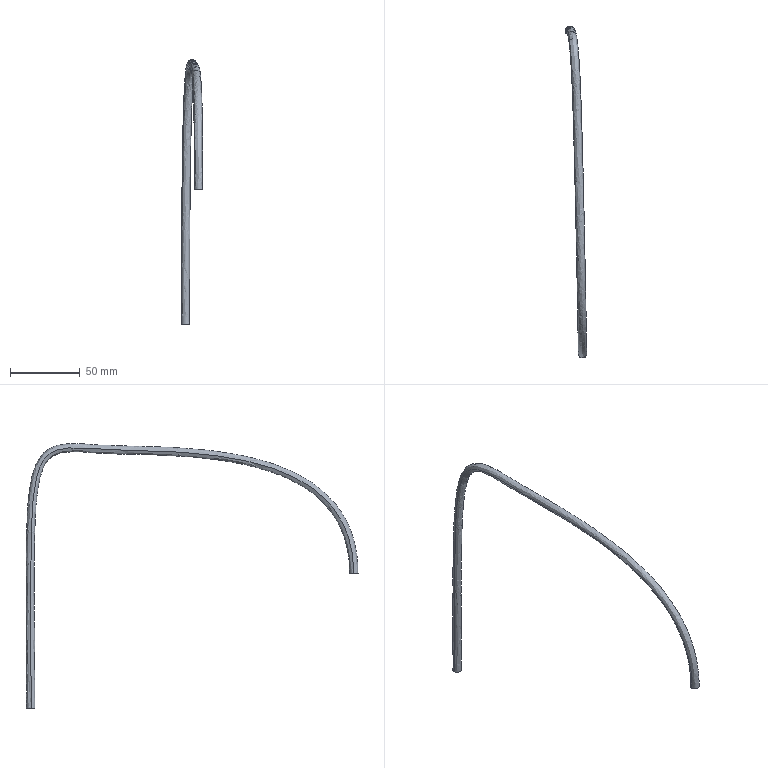Part | SolidWorks | features BaseBody 1 | 1 solid | 4 faces | box 15.406 x 237.723 x 189.724 mm | volume 12762 mm3 | spline 2 | plane 2
STEP:
#1=CARTESIAN_POINT('',(602.943,-193.052,343.045));
#2=VERTEX_POINT('',#1);
#3=CARTESIAN_POINT('',(596.944,-193.051,343.045));
#4=VERTEX_POINT('',#3);
#5=CARTESIAN_POINT('',(602.943,-193.052,343.045));
#6=CARTESIAN_POINT('',(602.943,-192.266,343.045));
#7=CARTESIAN_POINT('',(602.293,-190.702,343.045));
#8=CARTESIAN_POINT('',(599.943,-189.728,343.045));
#9=CARTESIAN_POINT('',(597.593,-190.702,343.045));
#10=CARTESIAN_POINT('',(596.944,-192.268,343.045));
#11=CARTESIAN_POINT('',(596.944,-193.051,343.045));
#12=B_SPLINE_CURVE_WITH_KNOTS('',3,(#5,#6,#7,#8,#9,#10,#11),.UNSPECIFIED.,.F.,.F.,(4,1,1,1,4),(0.009368,0.01171,0.01405,0.0164,0.01874),.UNSPECIFIED.);
#13=EDGE_CURVE('',#2,#4,#12,.T.);
#14=ORIENTED_EDGE('',*,*,#13,.T.);
#15=CARTESIAN_POINT('',(587.558,37.99,246.432));
#16=VERTEX_POINT('',#15);
#17=CARTESIAN_POINT('',(596.944,-193.051,343.045));
#18=CARTESIAN_POINT('',(596.944,-193.048,355.466));
#19=CARTESIAN_POINT('',(596.907,-190.885,366.117));
#20=CARTESIAN_POINT('',(596.772,-183.095,384.368));
#21=CARTESIAN_POINT('',(596.672,-177.485,391.983));
#22=CARTESIAN_POINT('',(596.422,-163.694,404.684));
#23=CARTESIAN_POINT('',(596.119,-147.351,414.874));
#24=CARTESIAN_POINT('',(595.344,-107.987,427.25));
#25=CARTESIAN_POINT('',(594.381,-63.958,430.712));
#26=CARTESIAN_POINT('',(593.449,-29.528,431.39));
#27=CARTESIAN_POINT('',(592.967,-14.614,431.839));
#28=CARTESIAN_POINT('',(592.728,-8.166,432.222));
#29=CARTESIAN_POINT('',(592.641,-5.946,432.39));
#30=CARTESIAN_POINT('',(592.61,-5.155,432.454));
#31=CARTESIAN_POINT('',(592.594,-4.765,432.487));
#32=CARTESIAN_POINT('',(592.334,1.621,433.044));
#33=CARTESIAN_POINT('',(591.933,9.581,433.39));
#34=CARTESIAN_POINT('',(591.378,17.891,432.117));
#35=CARTESIAN_POINT('',(590.956,23.07,430.097));
#36=CARTESIAN_POINT('',(590.535,27.306,426.808));
#37=CARTESIAN_POINT('',(590.118,30.703,422.03));
#38=CARTESIAN_POINT('',(589.575,34.228,413.383));
#39=CARTESIAN_POINT('',(589.193,35.866,404.037));
#40=CARTESIAN_POINT('',(588.607,37.778,384.601));
#41=CARTESIAN_POINT('',(588.299,38.193,369.487));
#42=CARTESIAN_POINT('',(587.905,38.355,336.976));
#43=CARTESIAN_POINT('',(587.652,38.205,307.087));
#44=CARTESIAN_POINT('',(587.558,37.99,268.306));
#45=CARTESIAN_POINT('',(587.558,37.99,246.432));
#46=B_SPLINE_CURVE_WITH_KNOTS('',3,(#17,#18,#19,#20,#21,#22,#23,#24,#25,#26,#27,#28,#29,#30,#31,#32,#33,#34,#35,#36,#37,#38,#39,#40,#41,#42,#43,#44,#45),.UNSPECIFIED.,.F.,.F.,(4,2,2,1,1,1,1,1,1,1,1,2,1,1,1,1,1,1,2,2,1,4),(0.,0.0625,0.125,0.1875,0.25,0.375,0.4375,0.4766,0.4922,0.4961,0.498,0.5,0.5625,0.5938,0.625,0.6562,0.6875,0.7188,0.7812,0.875,0.9375,1.),.UNSPECIFIED.);
#47=EDGE_CURVE('',#4,#16,#46,.T.);
#48=ORIENTED_EDGE('',*,*,#47,.T.);
#49=CARTESIAN_POINT('',(593.513,38.709,246.432));
#50=VERTEX_POINT('',#49);
#51=CARTESIAN_POINT('',(587.558,37.99,246.432));
#52=CARTESIAN_POINT('',(587.652,37.212,246.432));
#53=CARTESIAN_POINT('',(588.484,35.735,246.432));
#54=CARTESIAN_POINT('',(590.934,35.05,246.432));
#55=CARTESIAN_POINT('',(593.15,36.298,246.432));
#56=CARTESIAN_POINT('',(593.608,37.93,246.432));
#57=CARTESIAN_POINT('',(593.513,38.709,246.432));
#58=B_SPLINE_CURVE_WITH_KNOTS('',3,(#51,#52,#53,#54,#55,#56,#57),.UNSPECIFIED.,.F.,.F.,(4,1,1,1,4),(0.009368,0.01171,0.01405,0.0164,0.01874),.UNSPECIFIED.);
#59=EDGE_CURVE('',#16,#50,#58,.T.);
#60=ORIENTED_EDGE('',*,*,#59,.T.);
#61=CARTESIAN_POINT('',(602.943,-193.052,343.045));
#62=CARTESIAN_POINT('',(602.943,-193.048,355.478));
#63=CARTESIAN_POINT('',(602.906,-190.883,366.144));
#64=CARTESIAN_POINT('',(602.77,-183.081,384.424));
#65=CARTESIAN_POINT('',(602.671,-177.461,392.052));
#66=CARTESIAN_POINT('',(602.42,-163.647,404.773));
#67=CARTESIAN_POINT('',(602.116,-147.282,414.978));
#68=CARTESIAN_POINT('',(601.341,-107.88,427.364));
#69=CARTESIAN_POINT('',(600.377,-63.823,430.829));
#70=CARTESIAN_POINT('',(599.444,-29.358,431.508));
#71=CARTESIAN_POINT('',(598.961,-14.416,431.957));
#72=CARTESIAN_POINT('',(598.722,-7.948,432.341));
#73=CARTESIAN_POINT('',(598.635,-5.719,432.51));
#74=CARTESIAN_POINT('',(598.603,-4.925,432.574));
#75=CARTESIAN_POINT('',(598.587,-4.533,432.608));
#76=CARTESIAN_POINT('',(598.326,1.89,433.168));
#77=CARTESIAN_POINT('',(597.922,9.916,433.52));
#78=CARTESIAN_POINT('',(597.358,18.357,432.229));
#79=CARTESIAN_POINT('',(596.927,23.646,430.168));
#80=CARTESIAN_POINT('',(596.497,27.97,426.809));
#81=CARTESIAN_POINT('',(596.074,31.409,421.965));
#82=CARTESIAN_POINT('',(595.529,34.951,413.27));
#83=CARTESIAN_POINT('',(595.148,36.587,403.924));
#84=CARTESIAN_POINT('',(594.561,38.498,384.498));
#85=CARTESIAN_POINT('',(594.254,38.912,369.401));
#86=CARTESIAN_POINT('',(593.86,39.075,336.919));
#87=CARTESIAN_POINT('',(593.608,38.925,307.053));
#88=CARTESIAN_POINT('',(593.514,38.71,268.295));
#89=CARTESIAN_POINT('',(593.513,38.709,246.432));
#90=B_SPLINE_CURVE_WITH_KNOTS('',3,(#61,#62,#63,#64,#65,#66,#67,#68,#69,#70,#71,#72,#73,#74,#75,#76,#77,#78,#79,#80,#81,#82,#83,#84,#85,#86,#87,#88,#89),.UNSPECIFIED.,.F.,.F.,(4,2,2,1,1,1,1,1,1,1,1,2,1,1,1,1,1,1,2,2,1,4),(0.,0.0625,0.125,0.1875,0.25,0.375,0.4375,0.4766,0.4922,0.4961,0.498,0.5,0.5625,0.5938,0.625,0.6562,0.6875,0.7188,0.7812,0.875,0.9375,1.),.UNSPECIFIED.);
#91=EDGE_CURVE('',#2,#50,#90,.T.);
#92=ORIENTED_EDGE('',*,*,#91,.F.);
#93=EDGE_LOOP('',(#14,#48,#60,#92));
#94=FACE_OUTER_BOUND('',#93,.T.);
#95=CARTESIAN_POINT('',(602.943,-193.052,343.045));
#96=CARTESIAN_POINT('',(602.943,-193.048,355.478));
#97=CARTESIAN_POINT('',(602.906,-190.883,366.144));
#98=CARTESIAN_POINT('',(602.77,-183.081,384.424));
#99=CARTESIAN_POINT('',(602.671,-177.461,392.052));
#100=CARTESIAN_POINT('',(602.42,-163.647,404.773));
#101=CARTESIAN_POINT('',(602.116,-147.282,414.978));
#102=CARTESIAN_POINT('',(601.341,-107.88,427.364));
#103=CARTESIAN_POINT('',(600.377,-63.823,430.829));
#104=CARTESIAN_POINT('',(599.444,-29.358,431.508));
#105=CARTESIAN_POINT('',(598.961,-14.416,431.957));
#106=CARTESIAN_POINT('',(598.722,-7.948,432.341));
#107=CARTESIAN_POINT('',(598.635,-5.719,432.51));
#108=CARTESIAN_POINT('',(598.603,-4.925,432.574));
#109=CARTESIAN_POINT('',(598.587,-4.533,432.608));
#110=CARTESIAN_POINT('',(598.326,1.89,433.168));
#111=CARTESIAN_POINT('',(597.922,9.916,433.52));
#112=CARTESIAN_POINT('',(597.358,18.357,432.229));
#113=CARTESIAN_POINT('',(596.927,23.646,430.168));
#114=CARTESIAN_POINT('',(596.497,27.97,426.809));
#115=CARTESIAN_POINT('',(596.074,31.409,421.965));
#116=CARTESIAN_POINT('',(595.529,34.951,413.27));
#117=CARTESIAN_POINT('',(595.148,36.587,403.924));
#118=CARTESIAN_POINT('',(594.561,38.498,384.498));
#119=CARTESIAN_POINT('',(594.254,38.912,369.401));
#120=CARTESIAN_POINT('',(593.86,39.075,336.919));
#121=CARTESIAN_POINT('',(593.608,38.925,307.053));
#122=CARTESIAN_POINT('',(593.514,38.71,268.295));
#123=CARTESIAN_POINT('',(593.513,38.709,246.432));
#124=CARTESIAN_POINT('',(602.943,-192.266,343.045));
#125=CARTESIAN_POINT('',(602.943,-192.263,355.386));
#126=CARTESIAN_POINT('',(602.907,-190.115,365.941));
#127=CARTESIAN_POINT('',(602.772,-182.404,384.01));
#128=CARTESIAN_POINT('',(602.674,-176.855,391.543));
#129=CARTESIAN_POINT('',(602.425,-163.189,404.128));
#130=CARTESIAN_POINT('',(602.125,-146.968,414.249));
#131=CARTESIAN_POINT('',(601.354,-107.762,426.581));
#132=CARTESIAN_POINT('',(600.392,-63.79,430.044));
#133=CARTESIAN_POINT('',(599.459,-29.344,430.723));
#134=CARTESIAN_POINT('',(598.976,-14.385,431.172));
#135=CARTESIAN_POINT('',(598.736,-7.896,431.558));
#136=CARTESIAN_POINT('',(598.648,-5.658,431.727));
#137=CARTESIAN_POINT('',(598.616,-4.86,431.792));
#138=CARTESIAN_POINT('',(598.6,-4.464,431.826));
#139=CARTESIAN_POINT('',(598.34,1.94,432.384));
#140=CARTESIAN_POINT('',(597.938,9.912,432.729));
#141=CARTESIAN_POINT('',(597.386,18.17,431.46));
#142=CARTESIAN_POINT('',(596.971,23.264,429.47));
#143=CARTESIAN_POINT('',(596.56,27.392,426.263));
#144=CARTESIAN_POINT('',(596.153,30.712,421.598));
#145=CARTESIAN_POINT('',(595.618,34.184,413.089));
#146=CARTESIAN_POINT('',(595.239,35.815,403.813));
#147=CARTESIAN_POINT('',(594.655,37.717,384.467));
#148=CARTESIAN_POINT('',(594.348,38.133,369.387));
#149=CARTESIAN_POINT('',(593.954,38.295,336.92));
#150=CARTESIAN_POINT('',(593.702,38.145,307.059));
#151=CARTESIAN_POINT('',(593.608,37.93,268.298));
#152=CARTESIAN_POINT('',(593.608,37.93,246.432));
#153=CARTESIAN_POINT('',(602.293,-190.702,343.045));
#154=CARTESIAN_POINT('',(602.293,-190.698,355.203));
#155=CARTESIAN_POINT('',(602.257,-188.586,365.536));
#156=CARTESIAN_POINT('',(602.126,-181.056,383.18));
#157=CARTESIAN_POINT('',(602.03,-175.651,390.52));
#158=CARTESIAN_POINT('',(601.787,-162.28,402.833));
#159=CARTESIAN_POINT('',(601.492,-146.352,412.786));
#160=CARTESIAN_POINT('',(600.729,-107.538,425.007));
#161=CARTESIAN_POINT('',(599.771,-63.74,428.469));
#162=CARTESIAN_POINT('',(598.84,-29.334,429.146));
#163=CARTESIAN_POINT('',(598.355,-14.346,429.596));
#164=CARTESIAN_POINT('',(598.114,-7.817,429.984));
#165=CARTESIAN_POINT('',(598.025,-5.559,430.155));
#166=CARTESIAN_POINT('',(597.993,-4.756,430.22));
#167=CARTESIAN_POINT('',(597.977,-4.351,430.254));
#168=CARTESIAN_POINT('',(597.718,2.011,430.809));
#169=CARTESIAN_POINT('',(597.321,9.868,431.138));
#170=CARTESIAN_POINT('',(596.793,17.749,429.916));
#171=CARTESIAN_POINT('',(596.411,22.44,428.071));
#172=CARTESIAN_POINT('',(596.04,26.169,425.175));
#173=CARTESIAN_POINT('',(595.663,29.245,420.873));
#174=CARTESIAN_POINT('',(595.151,32.579,412.74));
#175=CARTESIAN_POINT('',(594.776,34.197,403.603));
#176=CARTESIAN_POINT('',(594.197,36.084,384.416));
#177=CARTESIAN_POINT('',(593.89,36.501,369.368));
#178=CARTESIAN_POINT('',(593.497,36.664,336.929));
#179=CARTESIAN_POINT('',(593.245,36.514,307.073));
#180=CARTESIAN_POINT('',(593.15,36.299,268.304));
#181=CARTESIAN_POINT('',(593.15,36.298,246.432));
#182=CARTESIAN_POINT('',(599.943,-189.728,343.045));
#183=CARTESIAN_POINT('',(599.943,-189.725,355.085));
#184=CARTESIAN_POINT('',(599.908,-187.636,365.275));
#185=CARTESIAN_POINT('',(599.778,-180.222,382.645));
#186=CARTESIAN_POINT('',(599.684,-174.91,389.861));
#187=CARTESIAN_POINT('',(599.445,-161.73,401.998));
#188=CARTESIAN_POINT('',(599.153,-145.991,411.841));
#189=CARTESIAN_POINT('',(598.395,-107.434,423.991));
#190=CARTESIAN_POINT('',(597.44,-63.753,427.451));
#191=CARTESIAN_POINT('',(596.51,-29.384,428.127));
#192=CARTESIAN_POINT('',(596.025,-14.386,428.577));
#193=CARTESIAN_POINT('',(595.783,-7.839,428.966));
#194=CARTESIAN_POINT('',(595.694,-5.572,429.137));
#195=CARTESIAN_POINT('',(595.662,-4.766,429.203));
#196=CARTESIAN_POINT('',(595.645,-4.355,429.238));
#197=CARTESIAN_POINT('',(595.388,1.968,429.789));
#198=CARTESIAN_POINT('',(594.995,9.731,430.107));
#199=CARTESIAN_POINT('',(594.485,17.336,428.919));
#200=CARTESIAN_POINT('',(594.126,21.741,427.178));
#201=CARTESIAN_POINT('',(593.782,25.192,424.499));
#202=CARTESIAN_POINT('',(593.426,28.104,420.442));
#203=CARTESIAN_POINT('',(592.929,31.345,412.559));
#204=CARTESIAN_POINT('',(592.557,32.957,403.51));
#205=CARTESIAN_POINT('',(591.981,34.835,384.417));
#206=CARTESIAN_POINT('',(591.674,35.253,369.383));
#207=CARTESIAN_POINT('',(591.281,35.415,336.953));
#208=CARTESIAN_POINT('',(591.028,35.266,307.093));
#209=CARTESIAN_POINT('',(590.934,35.05,268.311));
#210=CARTESIAN_POINT('',(590.934,35.05,246.432));
#211=CARTESIAN_POINT('',(597.593,-190.702,343.045));
#212=CARTESIAN_POINT('',(597.593,-190.698,355.193));
#213=CARTESIAN_POINT('',(597.557,-188.588,365.515));
#214=CARTESIAN_POINT('',(597.426,-181.067,383.136));
#215=CARTESIAN_POINT('',(597.331,-175.67,390.465));
#216=CARTESIAN_POINT('',(597.088,-162.317,402.763));
#217=CARTESIAN_POINT('',(596.793,-146.407,412.704));
#218=CARTESIAN_POINT('',(596.03,-107.622,424.917));
#219=CARTESIAN_POINT('',(595.073,-63.847,428.378));
#220=CARTESIAN_POINT('',(594.143,-29.468,429.054));
#221=CARTESIAN_POINT('',(593.659,-14.502,429.504));
#222=CARTESIAN_POINT('',(593.418,-7.989,429.89));
#223=CARTESIAN_POINT('',(593.33,-5.737,430.06));
#224=CARTESIAN_POINT('',(593.298,-4.937,430.125));
#225=CARTESIAN_POINT('',(593.281,-4.532,430.16));
#226=CARTESIAN_POINT('',(593.024,1.8,430.712));
#227=CARTESIAN_POINT('',(592.629,9.605,431.037));
#228=CARTESIAN_POINT('',(592.108,17.384,429.828));
#229=CARTESIAN_POINT('',(591.732,21.989,428.015));
#230=CARTESIAN_POINT('',(591.369,25.648,425.175));
#231=CARTESIAN_POINT('',(590.996,28.692,420.923));
#232=CARTESIAN_POINT('',(590.486,32.012,412.828));
#233=CARTESIAN_POINT('',(590.111,33.632,403.692));
#234=CARTESIAN_POINT('',(589.532,35.52,384.496));
#235=CARTESIAN_POINT('',(589.225,35.938,369.435));
#236=CARTESIAN_POINT('',(588.831,36.1,336.974));
#237=CARTESIAN_POINT('',(588.579,35.95,307.1));
#238=CARTESIAN_POINT('',(588.484,35.735,268.312));
#239=CARTESIAN_POINT('',(588.484,35.735,246.432));
#240=CARTESIAN_POINT('',(596.619,-193.051,343.045));
#241=CARTESIAN_POINT('',(596.619,-193.048,355.465));
#242=CARTESIAN_POINT('',(596.583,-190.885,366.116));
#243=CARTESIAN_POINT('',(596.447,-183.096,384.365));
#244=CARTESIAN_POINT('',(596.348,-177.487,391.979));
#245=CARTESIAN_POINT('',(596.097,-163.696,404.679));
#246=CARTESIAN_POINT('',(595.794,-147.355,414.869));
#247=CARTESIAN_POINT('',(595.02,-107.993,427.243));
#248=CARTESIAN_POINT('',(594.057,-63.965,430.705));
#249=CARTESIAN_POINT('',(593.125,-29.537,431.384));
#250=CARTESIAN_POINT('',(592.643,-14.625,431.833));
#251=CARTESIAN_POINT('',(592.404,-8.178,432.215));
#252=CARTESIAN_POINT('',(592.317,-5.959,432.383));
#253=CARTESIAN_POINT('',(592.286,-5.168,432.448));
#254=CARTESIAN_POINT('',(592.27,-4.778,432.481));
#255=CARTESIAN_POINT('',(592.01,1.607,433.038));
#256=CARTESIAN_POINT('',(591.61,9.563,433.383));
#257=CARTESIAN_POINT('',(591.054,17.866,432.11));
#258=CARTESIAN_POINT('',(590.633,23.039,430.093));
#259=CARTESIAN_POINT('',(590.212,27.27,426.808));
#260=CARTESIAN_POINT('',(589.795,30.664,422.033));
#261=CARTESIAN_POINT('',(589.253,34.189,413.389));
#262=CARTESIAN_POINT('',(588.871,35.827,404.043));
#263=CARTESIAN_POINT('',(588.285,37.739,384.606));
#264=CARTESIAN_POINT('',(587.977,38.154,369.492));
#265=CARTESIAN_POINT('',(587.583,38.316,336.979));
#266=CARTESIAN_POINT('',(587.33,38.166,307.089));
#267=CARTESIAN_POINT('',(587.236,37.951,268.307));
#268=CARTESIAN_POINT('',(587.236,37.951,246.432));
#269=CARTESIAN_POINT('',(597.593,-195.401,343.045));
#270=CARTESIAN_POINT('',(597.593,-195.398,355.741));
#271=CARTESIAN_POINT('',(597.555,-193.182,366.725));
#272=CARTESIAN_POINT('',(597.415,-185.12,385.613));
#273=CARTESIAN_POINT('',(597.312,-179.295,393.516));
#274=CARTESIAN_POINT('',(597.053,-165.061,406.624));
#275=CARTESIAN_POINT('',(596.742,-148.281,417.067));
#276=CARTESIAN_POINT('',(595.956,-108.329,429.607));
#277=CARTESIAN_POINT('',(594.986,-64.04,433.071));
#278=CARTESIAN_POINT('',(594.053,-29.552,433.752));
#279=CARTESIAN_POINT('',(593.572,-14.684,434.2));
#280=CARTESIAN_POINT('',(593.336,-8.297,434.579));
#281=CARTESIAN_POINT('',(593.25,-6.106,434.745));
#282=CARTESIAN_POINT('',(593.219,-5.324,434.809));
#283=CARTESIAN_POINT('',(593.203,-4.948,434.841));
#284=CARTESIAN_POINT('',(592.941,1.5,435.403));
#285=CARTESIAN_POINT('',(592.533,9.63,435.772));
#286=CARTESIAN_POINT('',(591.941,18.499,434.43));
#287=CARTESIAN_POINT('',(591.472,24.276,432.193));
#288=CARTESIAN_POINT('',(590.991,29.106,428.442));
#289=CARTESIAN_POINT('',(590.528,32.867,423.122));
#290=CARTESIAN_POINT('',(589.952,36.6,413.913));
#291=CARTESIAN_POINT('',(589.564,38.256,404.357));
#292=CARTESIAN_POINT('',(588.97,40.191,384.683));
#293=CARTESIAN_POINT('',(588.662,40.603,369.521));
#294=CARTESIAN_POINT('',(588.267,40.766,336.966));
#295=CARTESIAN_POINT('',(588.015,40.616,307.067));
#296=CARTESIAN_POINT('',(587.92,40.401,268.298));
#297=CARTESIAN_POINT('',(587.92,40.4,246.432));
#298=CARTESIAN_POINT('',(599.943,-196.375,343.045));
#299=CARTESIAN_POINT('',(599.943,-196.371,355.859));
#300=CARTESIAN_POINT('',(599.905,-194.132,366.986));
#301=CARTESIAN_POINT('',(599.762,-185.954,386.147));
#302=CARTESIAN_POINT('',(599.658,-180.037,394.175));
#303=CARTESIAN_POINT('',(599.395,-165.611,407.459));
#304=CARTESIAN_POINT('',(599.08,-148.641,418.011));
#305=CARTESIAN_POINT('',(598.29,-108.433,430.623));
#306=CARTESIAN_POINT('',(597.317,-64.027,434.089));
#307=CARTESIAN_POINT('',(596.383,-29.502,434.771));
#308=CARTESIAN_POINT('',(595.902,-14.643,435.219));
#309=CARTESIAN_POINT('',(595.666,-8.275,435.597));
#310=CARTESIAN_POINT('',(595.581,-6.094,435.762));
#311=CARTESIAN_POINT('',(595.55,-5.314,435.826));
#312=CARTESIAN_POINT('',(595.535,-4.943,435.857));
#313=CARTESIAN_POINT('',(595.271,1.544,436.423));
#314=CARTESIAN_POINT('',(594.859,9.766,436.803));
#315=CARTESIAN_POINT('',(594.249,18.912,435.427));
#316=CARTESIAN_POINT('',(593.757,24.975,433.086));
#317=CARTESIAN_POINT('',(593.248,30.083,429.119));
#318=CARTESIAN_POINT('',(592.764,34.008,423.552));
#319=CARTESIAN_POINT('',(592.173,37.834,414.094));
#320=CARTESIAN_POINT('',(591.783,39.496,404.45));
#321=CARTESIAN_POINT('',(591.186,41.441,384.682));
#322=CARTESIAN_POINT('',(590.878,41.851,369.505));
#323=CARTESIAN_POINT('',(590.483,42.014,336.942));
#324=CARTESIAN_POINT('',(590.231,41.864,307.047));
#325=CARTESIAN_POINT('',(590.136,41.649,268.291));
#326=CARTESIAN_POINT('',(590.136,41.649,246.432));
#327=CARTESIAN_POINT('',(602.293,-195.401,343.045));
#328=CARTESIAN_POINT('',(602.293,-195.398,355.75));
#329=CARTESIAN_POINT('',(602.255,-193.18,366.746));
#330=CARTESIAN_POINT('',(602.114,-185.109,385.656));
#331=CARTESIAN_POINT('',(602.011,-179.276,393.57));
#332=CARTESIAN_POINT('',(601.752,-165.025,406.694));
#333=CARTESIAN_POINT('',(601.441,-148.226,417.148));
#334=CARTESIAN_POINT('',(600.654,-108.245,429.697));
#335=CARTESIAN_POINT('',(599.684,-63.934,433.163));
#336=CARTESIAN_POINT('',(598.75,-29.418,433.844));
#337=CARTESIAN_POINT('',(598.268,-14.528,434.293));
#338=CARTESIAN_POINT('',(598.031,-8.126,434.673));
#339=CARTESIAN_POINT('',(597.945,-5.928,434.839));
#340=CARTESIAN_POINT('',(597.914,-5.144,434.903));
#341=CARTESIAN_POINT('',(597.899,-4.766,434.935));
#342=CARTESIAN_POINT('',(597.635,1.711,435.5));
#343=CARTESIAN_POINT('',(597.225,9.892,435.873));
#344=CARTESIAN_POINT('',(596.626,18.864,434.517));
#345=CARTESIAN_POINT('',(596.15,24.727,432.249));
#346=CARTESIAN_POINT('',(595.662,29.627,428.442));
#347=CARTESIAN_POINT('',(595.195,33.42,423.072));
#348=CARTESIAN_POINT('',(594.616,37.167,413.825));
#349=CARTESIAN_POINT('',(594.229,38.821,404.268));
#350=CARTESIAN_POINT('',(593.635,40.756,384.603));
#351=CARTESIAN_POINT('',(593.327,41.167,369.454));
#352=CARTESIAN_POINT('',(592.933,41.33,336.921));
#353=CARTESIAN_POINT('',(592.681,41.18,307.04));
#354=CARTESIAN_POINT('',(592.586,40.965,268.289));
#355=CARTESIAN_POINT('',(592.586,40.964,246.432));
#356=CARTESIAN_POINT('',(602.943,-193.837,343.045));
#357=CARTESIAN_POINT('',(602.943,-193.833,355.569));
#358=CARTESIAN_POINT('',(602.906,-191.65,366.346));
#359=CARTESIAN_POINT('',(602.768,-183.758,384.838));
#360=CARTESIAN_POINT('',(602.668,-178.067,392.562));
#361=CARTESIAN_POINT('',(602.414,-164.106,405.419));
#362=CARTESIAN_POINT('',(602.108,-147.595,415.707));
#363=CARTESIAN_POINT('',(601.329,-107.998,428.148));
#364=CARTESIAN_POINT('',(600.363,-63.855,431.613));
#365=CARTESIAN_POINT('',(599.429,-29.372,432.293));
#366=CARTESIAN_POINT('',(598.947,-14.446,432.742));
#367=CARTESIAN_POINT('',(598.708,-7.999,433.125));
#368=CARTESIAN_POINT('',(598.621,-5.781,433.293));
#369=CARTESIAN_POINT('',(598.59,-4.99,433.357));
#370=CARTESIAN_POINT('',(598.574,-4.602,433.39));
#371=CARTESIAN_POINT('',(598.312,1.84,433.952));
#372=CARTESIAN_POINT('',(597.906,9.921,434.311));
#373=CARTESIAN_POINT('',(597.33,18.543,432.998));
#374=CARTESIAN_POINT('',(596.884,24.028,430.866));
#375=CARTESIAN_POINT('',(596.434,28.548,427.355));
#376=CARTESIAN_POINT('',(595.996,32.107,422.333));
#377=CARTESIAN_POINT('',(595.44,35.718,413.452));
#378=CARTESIAN_POINT('',(595.056,37.36,404.035));
#379=CARTESIAN_POINT('',(594.468,39.279,384.53));
#380=CARTESIAN_POINT('',(594.16,39.692,369.416));
#381=CARTESIAN_POINT('',(593.766,39.854,336.918));
#382=CARTESIAN_POINT('',(593.514,39.704,307.048));
#383=CARTESIAN_POINT('',(593.419,39.489,268.293));
#384=CARTESIAN_POINT('',(593.419,39.489,246.432));
#385=CARTESIAN_POINT('',(602.943,-193.052,343.045));
#386=CARTESIAN_POINT('',(602.943,-193.048,355.478));
#387=CARTESIAN_POINT('',(602.906,-190.883,366.144));
#388=CARTESIAN_POINT('',(602.77,-183.081,384.424));
#389=CARTESIAN_POINT('',(602.671,-177.461,392.052));
#390=CARTESIAN_POINT('',(602.42,-163.647,404.773));
#391=CARTESIAN_POINT('',(602.116,-147.282,414.978));
#392=CARTESIAN_POINT('',(601.341,-107.88,427.364));
#393=CARTESIAN_POINT('',(600.377,-63.823,430.829));
#394=CARTESIAN_POINT('',(599.444,-29.358,431.508));
#395=CARTESIAN_POINT('',(598.961,-14.416,431.957));
#396=CARTESIAN_POINT('',(598.722,-7.948,432.341));
#397=CARTESIAN_POINT('',(598.635,-5.719,432.51));
#398=CARTESIAN_POINT('',(598.603,-4.925,432.574));
#399=CARTESIAN_POINT('',(598.587,-4.533,432.608));
#400=CARTESIAN_POINT('',(598.326,1.89,433.168));
#401=CARTESIAN_POINT('',(597.922,9.916,433.52));
#402=CARTESIAN_POINT('',(597.358,18.357,432.229));
#403=CARTESIAN_POINT('',(596.927,23.646,430.168));
#404=CARTESIAN_POINT('',(596.497,27.97,426.809));
#405=CARTESIAN_POINT('',(596.074,31.409,421.965));
#406=CARTESIAN_POINT('',(595.529,34.951,413.27));
#407=CARTESIAN_POINT('',(595.148,36.587,403.924));
#408=CARTESIAN_POINT('',(594.561,38.498,384.498));
#409=CARTESIAN_POINT('',(594.254,38.912,369.401));
#410=CARTESIAN_POINT('',(593.86,39.075,336.919));
#411=CARTESIAN_POINT('',(593.608,38.925,307.053));
#412=CARTESIAN_POINT('',(593.514,38.71,268.295));
#413=CARTESIAN_POINT('',(593.513,38.709,246.432));
#414=B_SPLINE_SURFACE_WITH_KNOTS('',3,3,((#95,#96,#97,#98,#99,#100,#101,#102,#103,#104,#105,#106,#107,#108,#109,#110,#111,#112,#113,#114,#115,#116,#117,#118,#119,#120,#121,#122,#123),(#124,#125,#126,#127,#128,#129,#130,#131,#132,#133,#134,#135,#136,#137,#138,#139,#140,#141,#142,#143,#144,#145,#146,#147,#148,#149,#150,#151,#152),(#153,#154,#155,#156,#157,#158,#159,#160,#161,#162,#163,#164,#165,#166,#167,#168,#169,#170,#171,#172,#173,#174,#175,#176,#177,#178,#179,#180,#181),(#182,#183,#184,#185,#186,#187,#188,#189,#190,#191,#192,#193,#194,#195,#196,#197,#198,#199,#200,#201,#202,#203,#204,#205,#206,#207,#208,#209,#210),(#211,#212,#213,#214,#215,#216,#217,#218,#219,#220,#221,#222,#223,#224,#225,#226,#227,#228,#229,#230,#231,#232,#233,#234,#235,#236,#237,#238,#239),(#240,#241,#242,#243,#244,#245,#246,#247,#248,#249,#250,#251,#252,#253,#254,#255,#256,#257,#258,#259,#260,#261,#262,#263,#264,#265,#266,#267,#268),(#269,#270,#271,#272,#273,#274,#275,#276,#277,#278,#279,#280,#281,#282,#283,#284,#285,#286,#287,#288,#289,#290,#291,#292,#293,#294,#295,#296,#297),(#298,#299,#300,#301,#302,#303,#304,#305,#306,#307,#308,#309,#310,#311,#312,#313,#314,#315,#316,#317,#318,#319,#320,#321,#322,#323,#324,#325,#326),(#327,#328,#329,#330,#331,#332,#333,#334,#335,#336,#337,#338,#339,#340,#341,#342,#343,#344,#345,#346,#347,#348,#349,#350,#351,#352,#353,#354,#355),(#356,#357,#358,#359,#360,#361,#362,#363,#364,#365,#366,#367,#368,#369,#370,#371,#372,#373,#374,#375,#376,#377,#378,#379,#380,#381,#382,#383,#384),(#385,#386,#387,#388,#389,#390,#391,#392,#393,#394,#395,#396,#397,#398,#399,#400,#401,#402,#403,#404,#405,#406,#407,#408,#409,#410,#411,#412,#413)),.UNSPECIFIED.,.T.,.F.,.F.,(4,1,1,1,1,1,1,1,4),(4,2,2,1,1,1,1,1,1,1,1,2,1,1,1,1,1,1,2,2,1,4),(0.,0.7854,1.571,2.356,3.142,3.927,4.712,5.498,6.283),(0.,0.0625,0.125,0.1875,0.25,0.375,0.4375,0.4766,0.4922,0.4961,0.498,0.5,0.5625,0.5938,0.625,0.6562,0.6875,0.7188,0.7812,0.875,0.9375,1.),.UNSPECIFIED.);
#415=ADVANCED_FACE('',(#94),#414,.T.);
#416=ORIENTED_EDGE('',*,*,#47,.F.);
#417=CARTESIAN_POINT('',(596.944,-193.051,343.045));
#418=CARTESIAN_POINT('',(596.944,-193.835,343.045));
#419=CARTESIAN_POINT('',(597.593,-195.401,343.045));
#420=CARTESIAN_POINT('',(599.943,-196.375,343.045));
#421=CARTESIAN_POINT('',(602.293,-195.401,343.045));
#422=CARTESIAN_POINT('',(602.943,-193.837,343.045));
#423=CARTESIAN_POINT('',(602.943,-193.052,343.045));
#424=B_SPLINE_CURVE_WITH_KNOTS('',3,(#417,#418,#419,#420,#421,#422,#423),.UNSPECIFIED.,.F.,.F.,(4,1,1,1,4),(0.01874,0.02108,0.02342,0.02576,0.02811),.UNSPECIFIED.);
#425=EDGE_CURVE('',#4,#2,#424,.T.);
#426=ORIENTED_EDGE('',*,*,#425,.T.);
#427=ORIENTED_EDGE('',*,*,#91,.T.);
#428=CARTESIAN_POINT('',(593.513,38.709,246.432));
#429=CARTESIAN_POINT('',(593.419,39.489,246.432));
#430=CARTESIAN_POINT('',(592.586,40.964,246.432));
#431=CARTESIAN_POINT('',(590.136,41.649,246.432));
#432=CARTESIAN_POINT('',(587.92,40.4,246.432));
#433=CARTESIAN_POINT('',(587.464,38.767,246.432));
#434=CARTESIAN_POINT('',(587.558,37.99,246.432));
#435=B_SPLINE_CURVE_WITH_KNOTS('',3,(#428,#429,#430,#431,#432,#433,#434),.UNSPECIFIED.,.F.,.F.,(4,1,1,1,4),(0.,0.002342,0.004684,0.007026,0.009368),.UNSPECIFIED.);
#436=EDGE_CURVE('',#50,#16,#435,.T.);
#437=ORIENTED_EDGE('',*,*,#436,.T.);
#438=EDGE_LOOP('',(#416,#426,#427,#437));
#439=FACE_OUTER_BOUND('',#438,.T.);
#440=CARTESIAN_POINT('',(602.943,-193.052,343.045));
#441=CARTESIAN_POINT('',(602.943,-193.048,355.478));
#442=CARTESIAN_POINT('',(602.906,-190.883,366.144));
#443=CARTESIAN_POINT('',(602.77,-183.081,384.424));
#444=CARTESIAN_POINT('',(602.671,-177.461,392.052));
#445=CARTESIAN_POINT('',(602.42,-163.647,404.773));
#446=CARTESIAN_POINT('',(602.116,-147.282,414.978));
#447=CARTESIAN_POINT('',(601.341,-107.88,427.364));
#448=CARTESIAN_POINT('',(600.377,-63.823,430.829));
#449=CARTESIAN_POINT('',(599.444,-29.358,431.508));
#450=CARTESIAN_POINT('',(598.961,-14.416,431.957));
#451=CARTESIAN_POINT('',(598.722,-7.948,432.341));
#452=CARTESIAN_POINT('',(598.635,-5.719,432.51));
#453=CARTESIAN_POINT('',(598.603,-4.925,432.574));
#454=CARTESIAN_POINT('',(598.587,-4.533,432.608));
#455=CARTESIAN_POINT('',(598.326,1.89,433.168));
#456=CARTESIAN_POINT('',(597.922,9.916,433.52));
#457=CARTESIAN_POINT('',(597.358,18.357,432.229));
#458=CARTESIAN_POINT('',(596.927,23.646,430.168));
#459=CARTESIAN_POINT('',(596.497,27.97,426.809));
#460=CARTESIAN_POINT('',(596.074,31.409,421.965));
#461=CARTESIAN_POINT('',(595.529,34.951,413.27));
#462=CARTESIAN_POINT('',(595.148,36.587,403.924));
#463=CARTESIAN_POINT('',(594.561,38.498,384.498));
#464=CARTESIAN_POINT('',(594.254,38.912,369.401));
#465=CARTESIAN_POINT('',(593.86,39.075,336.919));
#466=CARTESIAN_POINT('',(593.608,38.925,307.053));
#467=CARTESIAN_POINT('',(593.514,38.71,268.295));
#468=CARTESIAN_POINT('',(593.513,38.709,246.432));
#469=CARTESIAN_POINT('',(602.943,-192.266,343.045));
#470=CARTESIAN_POINT('',(602.943,-192.263,355.386));
#471=CARTESIAN_POINT('',(602.907,-190.115,365.941));
#472=CARTESIAN_POINT('',(602.772,-182.404,384.01));
#473=CARTESIAN_POINT('',(602.674,-176.855,391.543));
#474=CARTESIAN_POINT('',(602.425,-163.189,404.128));
#475=CARTESIAN_POINT('',(602.125,-146.968,414.249));
#476=CARTESIAN_POINT('',(601.354,-107.762,426.581));
#477=CARTESIAN_POINT('',(600.392,-63.79,430.044));
#478=CARTESIAN_POINT('',(599.459,-29.344,430.723));
#479=CARTESIAN_POINT('',(598.976,-14.385,431.172));
#480=CARTESIAN_POINT('',(598.736,-7.896,431.558));
#481=CARTESIAN_POINT('',(598.648,-5.658,431.727));
#482=CARTESIAN_POINT('',(598.616,-4.86,431.792));
#483=CARTESIAN_POINT('',(598.6,-4.464,431.826));
#484=CARTESIAN_POINT('',(598.34,1.94,432.384));
#485=CARTESIAN_POINT('',(597.938,9.912,432.729));
#486=CARTESIAN_POINT('',(597.386,18.17,431.46));
#487=CARTESIAN_POINT('',(596.971,23.264,429.47));
#488=CARTESIAN_POINT('',(596.56,27.392,426.263));
#489=CARTESIAN_POINT('',(596.153,30.712,421.598));
#490=CARTESIAN_POINT('',(595.618,34.184,413.089));
#491=CARTESIAN_POINT('',(595.239,35.815,403.813));
#492=CARTESIAN_POINT('',(594.655,37.717,384.467));
#493=CARTESIAN_POINT('',(594.348,38.133,369.387));
#494=CARTESIAN_POINT('',(593.954,38.295,336.92));
#495=CARTESIAN_POINT('',(593.702,38.145,307.059));
#496=CARTESIAN_POINT('',(593.608,37.93,268.298));
#497=CARTESIAN_POINT('',(593.608,37.93,246.432));
#498=CARTESIAN_POINT('',(602.293,-190.702,343.045));
#499=CARTESIAN_POINT('',(602.293,-190.698,355.203));
#500=CARTESIAN_POINT('',(602.257,-188.586,365.536));
#501=CARTESIAN_POINT('',(602.126,-181.056,383.18));
#502=CARTESIAN_POINT('',(602.03,-175.651,390.52));
#503=CARTESIAN_POINT('',(601.787,-162.28,402.833));
#504=CARTESIAN_POINT('',(601.492,-146.352,412.786));
#505=CARTESIAN_POINT('',(600.729,-107.538,425.007));
#506=CARTESIAN_POINT('',(599.771,-63.74,428.469));
#507=CARTESIAN_POINT('',(598.84,-29.334,429.146));
#508=CARTESIAN_POINT('',(598.355,-14.346,429.596));
#509=CARTESIAN_POINT('',(598.114,-7.817,429.984));
#510=CARTESIAN_POINT('',(598.025,-5.559,430.155));
#511=CARTESIAN_POINT('',(597.993,-4.756,430.22));
#512=CARTESIAN_POINT('',(597.977,-4.351,430.254));
#513=CARTESIAN_POINT('',(597.718,2.011,430.809));
#514=CARTESIAN_POINT('',(597.321,9.868,431.138));
#515=CARTESIAN_POINT('',(596.793,17.749,429.916));
#516=CARTESIAN_POINT('',(596.411,22.44,428.071));
#517=CARTESIAN_POINT('',(596.04,26.169,425.175));
#518=CARTESIAN_POINT('',(595.663,29.245,420.873));
#519=CARTESIAN_POINT('',(595.151,32.579,412.74));
#520=CARTESIAN_POINT('',(594.776,34.197,403.603));
#521=CARTESIAN_POINT('',(594.197,36.084,384.416));
#522=CARTESIAN_POINT('',(593.89,36.501,369.368));
#523=CARTESIAN_POINT('',(593.497,36.664,336.929));
#524=CARTESIAN_POINT('',(593.245,36.514,307.073));
#525=CARTESIAN_POINT('',(593.15,36.299,268.304));
#526=CARTESIAN_POINT('',(593.15,36.298,246.432));
#527=CARTESIAN_POINT('',(599.943,-189.728,343.045));
#528=CARTESIAN_POINT('',(599.943,-189.725,355.085));
#529=CARTESIAN_POINT('',(599.908,-187.636,365.275));
#530=CARTESIAN_POINT('',(599.778,-180.222,382.645));
#531=CARTESIAN_POINT('',(599.684,-174.91,389.861));
#532=CARTESIAN_POINT('',(599.445,-161.73,401.998));
#533=CARTESIAN_POINT('',(599.153,-145.991,411.841));
#534=CARTESIAN_POINT('',(598.395,-107.434,423.991));
#535=CARTESIAN_POINT('',(597.44,-63.753,427.451));
#536=CARTESIAN_POINT('',(596.51,-29.384,428.127));
#537=CARTESIAN_POINT('',(596.025,-14.386,428.577));
#538=CARTESIAN_POINT('',(595.783,-7.839,428.966));
#539=CARTESIAN_POINT('',(595.694,-5.572,429.137));
#540=CARTESIAN_POINT('',(595.662,-4.766,429.203));
#541=CARTESIAN_POINT('',(595.645,-4.355,429.238));
#542=CARTESIAN_POINT('',(595.388,1.968,429.789));
#543=CARTESIAN_POINT('',(594.995,9.731,430.107));
#544=CARTESIAN_POINT('',(594.485,17.336,428.919));
#545=CARTESIAN_POINT('',(594.126,21.741,427.178));
#546=CARTESIAN_POINT('',(593.782,25.192,424.499));
#547=CARTESIAN_POINT('',(593.426,28.104,420.442));
#548=CARTESIAN_POINT('',(592.929,31.345,412.559));
#549=CARTESIAN_POINT('',(592.557,32.957,403.51));
#550=CARTESIAN_POINT('',(591.981,34.835,384.417));
#551=CARTESIAN_POINT('',(591.674,35.253,369.383));
#552=CARTESIAN_POINT('',(591.281,35.415,336.953));
#553=CARTESIAN_POINT('',(591.028,35.266,307.093));
#554=CARTESIAN_POINT('',(590.934,35.05,268.311));
#555=CARTESIAN_POINT('',(590.934,35.05,246.432));
#556=CARTESIAN_POINT('',(597.593,-190.702,343.045));
#557=CARTESIAN_POINT('',(597.593,-190.698,355.193));
#558=CARTESIAN_POINT('',(597.557,-188.588,365.515));
#559=CARTESIAN_POINT('',(597.426,-181.067,383.136));
#560=CARTESIAN_POINT('',(597.331,-175.67,390.465));
#561=CARTESIAN_POINT('',(597.088,-162.317,402.763));
#562=CARTESIAN_POINT('',(596.793,-146.407,412.704));
#563=CARTESIAN_POINT('',(596.03,-107.622,424.917));
#564=CARTESIAN_POINT('',(595.073,-63.847,428.378));
#565=CARTESIAN_POINT('',(594.143,-29.468,429.054));
#566=CARTESIAN_POINT('',(593.659,-14.502,429.504));
#567=CARTESIAN_POINT('',(593.418,-7.989,429.89));
#568=CARTESIAN_POINT('',(593.33,-5.737,430.06));
#569=CARTESIAN_POINT('',(593.298,-4.937,430.125));
#570=CARTESIAN_POINT('',(593.281,-4.532,430.16));
#571=CARTESIAN_POINT('',(593.024,1.8,430.712));
#572=CARTESIAN_POINT('',(592.629,9.605,431.037));
#573=CARTESIAN_POINT('',(592.108,17.384,429.828));
#574=CARTESIAN_POINT('',(591.732,21.989,428.015));
#575=CARTESIAN_POINT('',(591.369,25.648,425.175));
#576=CARTESIAN_POINT('',(590.996,28.692,420.923));
#577=CARTESIAN_POINT('',(590.486,32.012,412.828));
#578=CARTESIAN_POINT('',(590.111,33.632,403.692));
#579=CARTESIAN_POINT('',(589.532,35.52,384.496));
#580=CARTESIAN_POINT('',(589.225,35.938,369.435));
#581=CARTESIAN_POINT('',(588.831,36.1,336.974));
#582=CARTESIAN_POINT('',(588.579,35.95,307.1));
#583=CARTESIAN_POINT('',(588.484,35.735,268.312));
#584=CARTESIAN_POINT('',(588.484,35.735,246.432));
#585=CARTESIAN_POINT('',(596.619,-193.051,343.045));
#586=CARTESIAN_POINT('',(596.619,-193.048,355.465));
#587=CARTESIAN_POINT('',(596.583,-190.885,366.116));
#588=CARTESIAN_POINT('',(596.447,-183.096,384.365));
#589=CARTESIAN_POINT('',(596.348,-177.487,391.979));
#590=CARTESIAN_POINT('',(596.097,-163.696,404.679));
#591=CARTESIAN_POINT('',(595.794,-147.355,414.869));
#592=CARTESIAN_POINT('',(595.02,-107.993,427.243));
#593=CARTESIAN_POINT('',(594.057,-63.965,430.705));
#594=CARTESIAN_POINT('',(593.125,-29.537,431.384));
#595=CARTESIAN_POINT('',(592.643,-14.625,431.833));
#596=CARTESIAN_POINT('',(592.404,-8.178,432.215));
#597=CARTESIAN_POINT('',(592.317,-5.959,432.383));
#598=CARTESIAN_POINT('',(592.286,-5.168,432.448));
#599=CARTESIAN_POINT('',(592.27,-4.778,432.481));
#600=CARTESIAN_POINT('',(592.01,1.607,433.038));
#601=CARTESIAN_POINT('',(591.61,9.563,433.383));
#602=CARTESIAN_POINT('',(591.054,17.866,432.11));
#603=CARTESIAN_POINT('',(590.633,23.039,430.093));
#604=CARTESIAN_POINT('',(590.212,27.27,426.808));
#605=CARTESIAN_POINT('',(589.795,30.664,422.033));
#606=CARTESIAN_POINT('',(589.253,34.189,413.389));
#607=CARTESIAN_POINT('',(588.871,35.827,404.043));
#608=CARTESIAN_POINT('',(588.285,37.739,384.606));
#609=CARTESIAN_POINT('',(587.977,38.154,369.492));
#610=CARTESIAN_POINT('',(587.583,38.316,336.979));
#611=CARTESIAN_POINT('',(587.33,38.166,307.089));
#612=CARTESIAN_POINT('',(587.236,37.951,268.307));
#613=CARTESIAN_POINT('',(587.236,37.951,246.432));
#614=CARTESIAN_POINT('',(597.593,-195.401,343.045));
#615=CARTESIAN_POINT('',(597.593,-195.398,355.741));
#616=CARTESIAN_POINT('',(597.555,-193.182,366.725));
#617=CARTESIAN_POINT('',(597.415,-185.12,385.613));
#618=CARTESIAN_POINT('',(597.312,-179.295,393.516));
#619=CARTESIAN_POINT('',(597.053,-165.061,406.624));
#620=CARTESIAN_POINT('',(596.742,-148.281,417.067));
#621=CARTESIAN_POINT('',(595.956,-108.329,429.607));
#622=CARTESIAN_POINT('',(594.986,-64.04,433.071));
#623=CARTESIAN_POINT('',(594.053,-29.552,433.752));
#624=CARTESIAN_POINT('',(593.572,-14.684,434.2));
#625=CARTESIAN_POINT('',(593.336,-8.297,434.579));
#626=CARTESIAN_POINT('',(593.25,-6.106,434.745));
#627=CARTESIAN_POINT('',(593.219,-5.324,434.809));
#628=CARTESIAN_POINT('',(593.203,-4.948,434.841));
#629=CARTESIAN_POINT('',(592.941,1.5,435.403));
#630=CARTESIAN_POINT('',(592.533,9.63,435.772));
#631=CARTESIAN_POINT('',(591.941,18.499,434.43));
#632=CARTESIAN_POINT('',(591.472,24.276,432.193));
#633=CARTESIAN_POINT('',(590.991,29.106,428.442));
#634=CARTESIAN_POINT('',(590.528,32.867,423.122));
#635=CARTESIAN_POINT('',(589.952,36.6,413.913));
#636=CARTESIAN_POINT('',(589.564,38.256,404.357));
#637=CARTESIAN_POINT('',(588.97,40.191,384.683));
#638=CARTESIAN_POINT('',(588.662,40.603,369.521));
#639=CARTESIAN_POINT('',(588.267,40.766,336.966));
#640=CARTESIAN_POINT('',(588.015,40.616,307.067));
#641=CARTESIAN_POINT('',(587.92,40.401,268.298));
#642=CARTESIAN_POINT('',(587.92,40.4,246.432));
#643=CARTESIAN_POINT('',(599.943,-196.375,343.045));
#644=CARTESIAN_POINT('',(599.943,-196.371,355.859));
#645=CARTESIAN_POINT('',(599.905,-194.132,366.986));
#646=CARTESIAN_POINT('',(599.762,-185.954,386.147));
#647=CARTESIAN_POINT('',(599.658,-180.037,394.175));
#648=CARTESIAN_POINT('',(599.395,-165.611,407.459));
#649=CARTESIAN_POINT('',(599.08,-148.641,418.011));
#650=CARTESIAN_POINT('',(598.29,-108.433,430.623));
#651=CARTESIAN_POINT('',(597.317,-64.027,434.089));
#652=CARTESIAN_POINT('',(596.383,-29.502,434.771));
#653=CARTESIAN_POINT('',(595.902,-14.643,435.219));
#654=CARTESIAN_POINT('',(595.666,-8.275,435.597));
#655=CARTESIAN_POINT('',(595.581,-6.094,435.762));
#656=CARTESIAN_POINT('',(595.55,-5.314,435.826));
#657=CARTESIAN_POINT('',(595.535,-4.943,435.857));
#658=CARTESIAN_POINT('',(595.271,1.544,436.423));
#659=CARTESIAN_POINT('',(594.859,9.766,436.803));
#660=CARTESIAN_POINT('',(594.249,18.912,435.427));
#661=CARTESIAN_POINT('',(593.757,24.975,433.086));
#662=CARTESIAN_POINT('',(593.248,30.083,429.119));
#663=CARTESIAN_POINT('',(592.764,34.008,423.552));
#664=CARTESIAN_POINT('',(592.173,37.834,414.094));
#665=CARTESIAN_POINT('',(591.783,39.496,404.45));
#666=CARTESIAN_POINT('',(591.186,41.441,384.682));
#667=CARTESIAN_POINT('',(590.878,41.851,369.505));
#668=CARTESIAN_POINT('',(590.483,42.014,336.942));
#669=CARTESIAN_POINT('',(590.231,41.864,307.047));
#670=CARTESIAN_POINT('',(590.136,41.649,268.291));
#671=CARTESIAN_POINT('',(590.136,41.649,246.432));
#672=CARTESIAN_POINT('',(602.293,-195.401,343.045));
#673=CARTESIAN_POINT('',(602.293,-195.398,355.75));
#674=CARTESIAN_POINT('',(602.255,-193.18,366.746));
#675=CARTESIAN_POINT('',(602.114,-185.109,385.656));
#676=CARTESIAN_POINT('',(602.011,-179.276,393.57));
#677=CARTESIAN_POINT('',(601.752,-165.025,406.694));
#678=CARTESIAN_POINT('',(601.441,-148.226,417.148));
#679=CARTESIAN_POINT('',(600.654,-108.245,429.697));
#680=CARTESIAN_POINT('',(599.684,-63.934,433.163));
#681=CARTESIAN_POINT('',(598.75,-29.418,433.844));
#682=CARTESIAN_POINT('',(598.268,-14.528,434.293));
#683=CARTESIAN_POINT('',(598.031,-8.126,434.673));
#684=CARTESIAN_POINT('',(597.945,-5.928,434.839));
#685=CARTESIAN_POINT('',(597.914,-5.144,434.903));
#686=CARTESIAN_POINT('',(597.899,-4.766,434.935));
#687=CARTESIAN_POINT('',(597.635,1.711,435.5));
#688=CARTESIAN_POINT('',(597.225,9.892,435.873));
#689=CARTESIAN_POINT('',(596.626,18.864,434.517));
#690=CARTESIAN_POINT('',(596.15,24.727,432.249));
#691=CARTESIAN_POINT('',(595.662,29.627,428.442));
#692=CARTESIAN_POINT('',(595.195,33.42,423.072));
#693=CARTESIAN_POINT('',(594.616,37.167,413.825));
#694=CARTESIAN_POINT('',(594.229,38.821,404.268));
#695=CARTESIAN_POINT('',(593.635,40.756,384.603));
#696=CARTESIAN_POINT('',(593.327,41.167,369.454));
#697=CARTESIAN_POINT('',(592.933,41.33,336.921));
#698=CARTESIAN_POINT('',(592.681,41.18,307.04));
#699=CARTESIAN_POINT('',(592.586,40.965,268.289));
#700=CARTESIAN_POINT('',(592.586,40.964,246.432));
#701=CARTESIAN_POINT('',(602.943,-193.837,343.045));
#702=CARTESIAN_POINT('',(602.943,-193.833,355.569));
#703=CARTESIAN_POINT('',(602.906,-191.65,366.346));
#704=CARTESIAN_POINT('',(602.768,-183.758,384.838));
#705=CARTESIAN_POINT('',(602.668,-178.067,392.562));
#706=CARTESIAN_POINT('',(602.414,-164.106,405.419));
#707=CARTESIAN_POINT('',(602.108,-147.595,415.707));
#708=CARTESIAN_POINT('',(601.329,-107.998,428.148));
#709=CARTESIAN_POINT('',(600.363,-63.855,431.613));
#710=CARTESIAN_POINT('',(599.429,-29.372,432.293));
#711=CARTESIAN_POINT('',(598.947,-14.446,432.742));
#712=CARTESIAN_POINT('',(598.708,-7.999,433.125));
#713=CARTESIAN_POINT('',(598.621,-5.781,433.293));
#714=CARTESIAN_POINT('',(598.59,-4.99,433.357));
#715=CARTESIAN_POINT('',(598.574,-4.602,433.39));
#716=CARTESIAN_POINT('',(598.312,1.84,433.952));
#717=CARTESIAN_POINT('',(597.906,9.921,434.311));
#718=CARTESIAN_POINT('',(597.33,18.543,432.998));
#719=CARTESIAN_POINT('',(596.884,24.028,430.866));
#720=CARTESIAN_POINT('',(596.434,28.548,427.355));
#721=CARTESIAN_POINT('',(595.996,32.107,422.333));
#722=CARTESIAN_POINT('',(595.44,35.718,413.452));
#723=CARTESIAN_POINT('',(595.056,37.36,404.035));
#724=CARTESIAN_POINT('',(594.468,39.279,384.53));
#725=CARTESIAN_POINT('',(594.16,39.692,369.416));
#726=CARTESIAN_POINT('',(593.766,39.854,336.918));
#727=CARTESIAN_POINT('',(593.514,39.704,307.048));
#728=CARTESIAN_POINT('',(593.419,39.489,268.293));
#729=CARTESIAN_POINT('',(593.419,39.489,246.432));
#730=CARTESIAN_POINT('',(602.943,-193.052,343.045));
#731=CARTESIAN_POINT('',(602.943,-193.048,355.478));
#732=CARTESIAN_POINT('',(602.906,-190.883,366.144));
#733=CARTESIAN_POINT('',(602.77,-183.081,384.424));
#734=CARTESIAN_POINT('',(602.671,-177.461,392.052));
#735=CARTESIAN_POINT('',(602.42,-163.647,404.773));
#736=CARTESIAN_POINT('',(602.116,-147.282,414.978));
#737=CARTESIAN_POINT('',(601.341,-107.88,427.364));
#738=CARTESIAN_POINT('',(600.377,-63.823,430.829));
#739=CARTESIAN_POINT('',(599.444,-29.358,431.508));
#740=CARTESIAN_POINT('',(598.961,-14.416,431.957));
#741=CARTESIAN_POINT('',(598.722,-7.948,432.341));
#742=CARTESIAN_POINT('',(598.635,-5.719,432.51));
#743=CARTESIAN_POINT('',(598.603,-4.925,432.574));
#744=CARTESIAN_POINT('',(598.587,-4.533,432.608));
#745=CARTESIAN_POINT('',(598.326,1.89,433.168));
#746=CARTESIAN_POINT('',(597.922,9.916,433.52));
#747=CARTESIAN_POINT('',(597.358,18.357,432.229));
#748=CARTESIAN_POINT('',(596.927,23.646,430.168));
#749=CARTESIAN_POINT('',(596.497,27.97,426.809));
#750=CARTESIAN_POINT('',(596.074,31.409,421.965));
#751=CARTESIAN_POINT('',(595.529,34.951,413.27));
#752=CARTESIAN_POINT('',(595.148,36.587,403.924));
#753=CARTESIAN_POINT('',(594.561,38.498,384.498));
#754=CARTESIAN_POINT('',(594.254,38.912,369.401));
#755=CARTESIAN_POINT('',(593.86,39.075,336.919));
#756=CARTESIAN_POINT('',(593.608,38.925,307.053));
#757=CARTESIAN_POINT('',(593.514,38.71,268.295));
#758=CARTESIAN_POINT('',(593.513,38.709,246.432));
#759=B_SPLINE_SURFACE_WITH_KNOTS('',3,3,((#440,#441,#442,#443,#444,#445,#446,#447,#448,#449,#450,#451,#452,#453,#454,#455,#456,#457,#458,#459,#460,#461,#462,#463,#464,#465,#466,#467,#468),(#469,#470,#471,#472,#473,#474,#475,#476,#477,#478,#479,#480,#481,#482,#483,#484,#485,#486,#487,#488,#489,#490,#491,#492,#493,#494,#495,#496,#497),(#498,#499,#500,#501,#502,#503,#504,#505,#506,#507,#508,#509,#510,#511,#512,#513,#514,#515,#516,#517,#518,#519,#520,#521,#522,#523,#524,#525,#526),(#527,#528,#529,#530,#531,#532,#533,#534,#535,#536,#537,#538,#539,#540,#541,#542,#543,#544,#545,#546,#547,#548,#549,#550,#551,#552,#553,#554,#555),(#556,#557,#558,#559,#560,#561,#562,#563,#564,#565,#566,#567,#568,#569,#570,#571,#572,#573,#574,#575,#576,#577,#578,#579,#580,#581,#582,#583,#584),(#585,#586,#587,#588,#589,#590,#591,#592,#593,#594,#595,#596,#597,#598,#599,#600,#601,#602,#603,#604,#605,#606,#607,#608,#609,#610,#611,#612,#613),(#614,#615,#616,#617,#618,#619,#620,#621,#622,#623,#624,#625,#626,#627,#628,#629,#630,#631,#632,#633,#634,#635,#636,#637,#638,#639,#640,#641,#642),(#643,#644,#645,#646,#647,#648,#649,#650,#651,#652,#653,#654,#655,#656,#657,#658,#659,#660,#661,#662,#663,#664,#665,#666,#667,#668,#669,#670,#671),(#672,#673,#674,#675,#676,#677,#678,#679,#680,#681,#682,#683,#684,#685,#686,#687,#688,#689,#690,#691,#692,#693,#694,#695,#696,#697,#698,#699,#700),(#701,#702,#703,#704,#705,#706,#707,#708,#709,#710,#711,#712,#713,#714,#715,#716,#717,#718,#719,#720,#721,#722,#723,#724,#725,#726,#727,#728,#729),(#730,#731,#732,#733,#734,#735,#736,#737,#738,#739,#740,#741,#742,#743,#744,#745,#746,#747,#748,#749,#750,#751,#752,#753,#754,#755,#756,#757,#758)),.UNSPECIFIED.,.T.,.F.,.F.,(4,1,1,1,1,1,1,1,4),(4,2,2,1,1,1,1,1,1,1,1,2,1,1,1,1,1,1,2,2,1,4),(0.,0.7854,1.571,2.356,3.142,3.927,4.712,5.498,6.283),(0.,0.0625,0.125,0.1875,0.25,0.375,0.4375,0.4766,0.4922,0.4961,0.498,0.5,0.5625,0.5938,0.625,0.6562,0.6875,0.7188,0.7812,0.875,0.9375,1.),.UNSPECIFIED.);
#760=ADVANCED_FACE('',(#439),#759,.T.);
#761=ORIENTED_EDGE('',*,*,#436,.F.);
#762=ORIENTED_EDGE('',*,*,#59,.F.);
#763=EDGE_LOOP('',(#761,#762));
#764=FACE_OUTER_BOUND('',#763,.T.);
#765=CARTESIAN_POINT('',(590.535,38.349,246.432));
#766=DIRECTION('',(0.,-0.000000024,-1.));
#767=DIRECTION('',(0.,1.,-0.000000024));
#768=AXIS2_PLACEMENT_3D('',#765,#766,#767);
#769=PLANE('',#768);
#770=ADVANCED_FACE('',(#764),#769,.T.);
#771=ORIENTED_EDGE('',*,*,#13,.F.);
#772=ORIENTED_EDGE('',*,*,#425,.F.);
#773=EDGE_LOOP('',(#771,#772));
#774=FACE_OUTER_BOUND('',#773,.T.);
#775=CARTESIAN_POINT('',(599.943,-193.052,343.045));
#776=DIRECTION('',(0.,0.,1.));
#777=DIRECTION('',(1.,0.,0.));
#778=AXIS2_PLACEMENT_3D('',#775,#776,#777);
#779=PLANE('',#778);
#780=ADVANCED_FACE('',(#774),#779,.F.);
#781=CLOSED_SHELL('',(#415,#760,#770,#780));
#782=MANIFOLD_SOLID_BREP('',#781);
#783=CARTESIAN_POINT('',(0.,0.,0.));
#784=DIRECTION('',(0.,0.,1.));
#785=DIRECTION('',(1.,0.,0.));
#786=AXIS2_PLACEMENT_3D('',#783,#784,#785);
#787=(LENGTH_UNIT()NAMED_UNIT(*)SI_UNIT(.MILLI.,.METRE.));
#788=UNCERTAINTY_MEASURE_WITH_UNIT(LENGTH_MEASURE(0.00001),#787,'','');
#789=(NAMED_UNIT(*)PLANE_ANGLE_UNIT()SI_UNIT($,.RADIAN.));
#790=(NAMED_UNIT(*)SI_UNIT($,.STERADIAN.)SOLID_ANGLE_UNIT());
#791=(GEOMETRIC_REPRESENTATION_CONTEXT(3)GLOBAL_UNCERTAINTY_ASSIGNED_CONTEXT((#788))GLOBAL_UNIT_ASSIGNED_CONTEXT((#787,#789,#790))REPRESENTATION_CONTEXT('',''));
#792=ADVANCED_BREP_SHAPE_REPRESENTATION('',(#782,#786),#791);